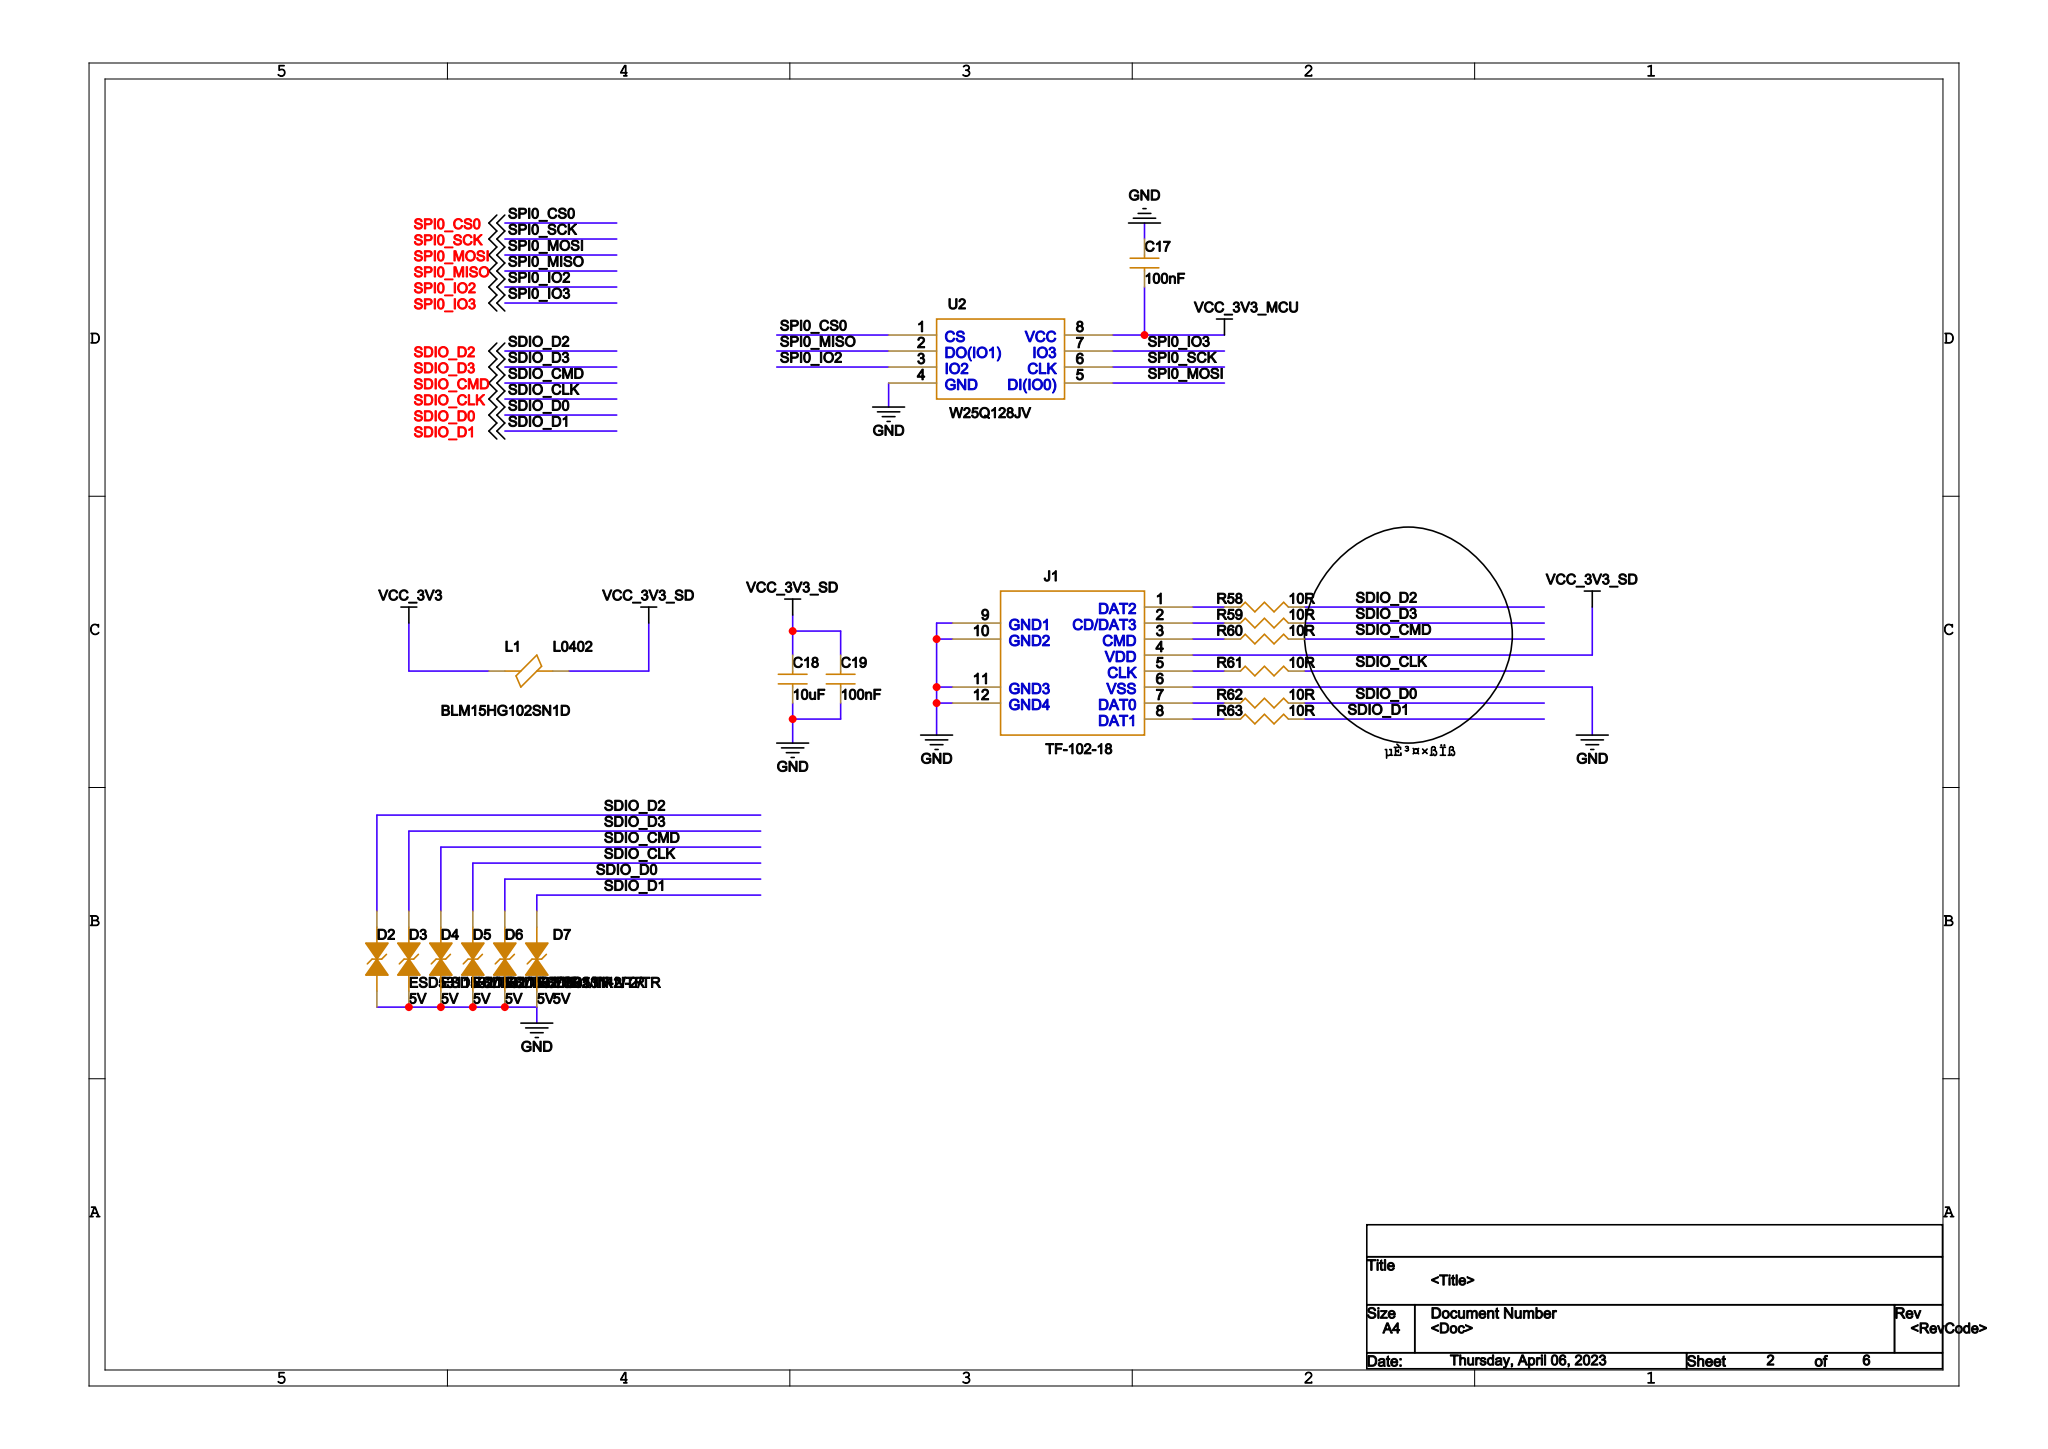Circuit board | Cadence Allegro | 278 parts | 154 nets | one sheet of the schematic
Parts on this sheet (reference | value | footprint):
C17 | 100nF | C0402
C18 | 10uF | C0603
C19 | 100nF | C0402
D2 | ESD5311N-2/TR | DFN1006-2L
D3 | ESD5311N-2/TR | DFN1006-2L
D4 | ESD5311N-2/TR | DFN1006-2L
D5 | ESD5311N-2/TR | DFN1006-2L
D6 | ESD5311N-2/TR | DFN1006-2L
D7 | ESD5311N-2/TR | DFN1006-2L
J1 | TF-102-18 | TF-102-18
L1 | BLM15HG102SN1D | L0402
R58 | 10R | R0402
R59 | 10R | R0402
R60 | 10R | R0402
R61 | 10R | R0402
R62 | 10R | R0402
R63 | 10R | R0402
U2 | W25Q128JV | SOIC-8-208MIL
Nets of these parts (net: part-pin ...):
GND: C17-2 C18-1 C19-1 D2-2 D3-2 D4-2 D5-2 D6-2 D7-2 J1-6 J1-9 J1-10 J1-11 J1-12 U2-4
SDIO_D2: D2-1 R58-2
SDIO_D3: D3-1 R59-2
SDIO_CMD: D4-1 R60-2
SDIO_CLK: D5-1 R61-2
SDIO_D0: D6-1 R62-2
SDIO_D1: D7-1 R63-2
VCC_3V3_MCU: C17-1 U2-8
VCC_3V3_SD: C18-2 C19-2 J1-4 L1-2
VCC_3V3: L1-1
N16770740: J1-2 R59-1
N16770728: J1-5 R61-1
N16770732: J1-3 R60-1
N16770744: J1-7 R62-1
N16770736: J1-8 R63-1
N16770706: J1-1 R58-1
SPI0_CS0: U2-1
SPI0_IO2: U2-3
SPI0_IO3: U2-7
SPI0_MISO: U2-2
SPI0_MOSI: U2-5
SPI0_SCK: U2-6